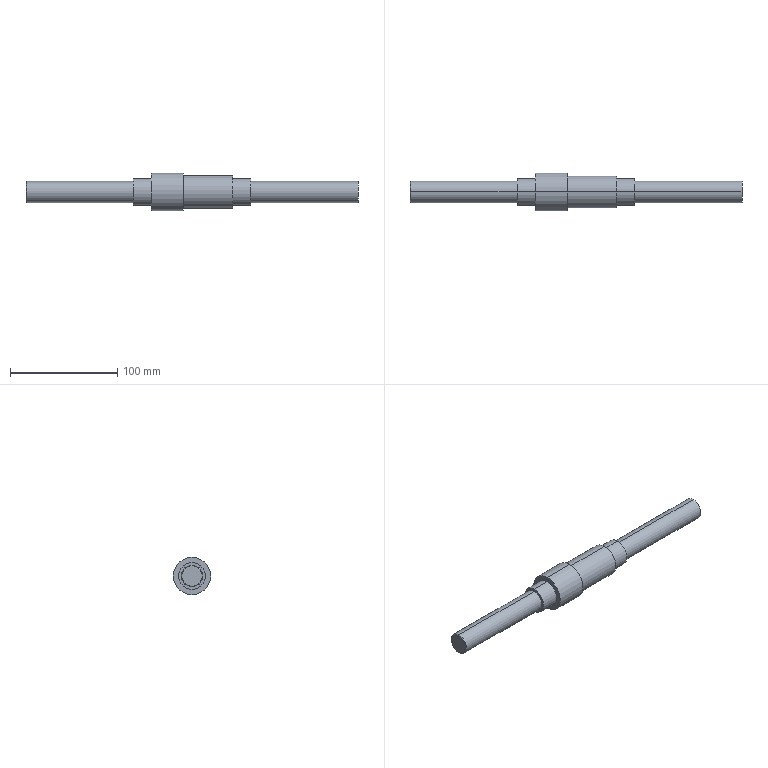Part | STEP file | 1 solid | 21 faces | box 310 x 35 x 35 mm | volume 140893 mm3 | cylinder 12 | plane 7 | cone 2 | commonest cylinder face diameters 20 x4 25 x4 30 x2 35 x2
STEP:
#1=CARTESIAN_POINT('',(0.,0.,0.));
#2=DIRECTION('',(0.,0.,1.));
#3=DIRECTION('',(1.,0.,0.));
#4=AXIS2_PLACEMENT_3D('',#1,#2,#3);
#5=CARTESIAN_POINT('',(210.,0.,-10.));
#6=VERTEX_POINT('',#5);
#7=CARTESIAN_POINT('',(210.,0.,10.));
#8=VERTEX_POINT('',#7);
#9=CARTESIAN_POINT('',(210.,0.,0.));
#10=DIRECTION('',(1.,0.,0.));
#11=DIRECTION('',(0.,0.,-1.));
#12=AXIS2_PLACEMENT_3D('',#9,#10,#11);
#13=CIRCLE('',#12,10.);
#14=CARTESIAN_POINT('',(260.,0.,0.));
#15=DIRECTION('',(1.,0.,0.));
#16=DIRECTION('',(0.,0.,-1.));
#17=AXIS2_PLACEMENT_3D('',#14,#15,#16);
#18=CYLINDRICAL_SURFACE('',#17,10.);
#19=CARTESIAN_POINT('',(0.,-50.));
#20=DIRECTION('',(1.,0.));
#21=VECTOR('',#20,1.);
#22=LINE('',#19,#21);
#23=(GEOMETRIC_REPRESENTATION_CONTEXT(2)PARAMETRIC_REPRESENTATION_CONTEXT()REPRESENTATION_CONTEXT('',''));
#24=DEFINITIONAL_REPRESENTATION('',(#22),#23);
#25=PCURVE('',#18,#24);
#26=CARTESIAN_POINT('',(210.,10.,0.));
#27=DIRECTION('',(1.,0.,0.));
#28=DIRECTION('',(0.,0.,-1.));
#29=AXIS2_PLACEMENT_3D('',#26,#27,#28);
#30=PLANE('',#29);
#31=CARTESIAN_POINT('',(0.,-10.));
#32=DIRECTION('',(1.,0.));
#33=AXIS2_PLACEMENT_2D('',#31,#32);
#34=CIRCLE('',#33,10.);
#35=(GEOMETRIC_REPRESENTATION_CONTEXT(2)PARAMETRIC_REPRESENTATION_CONTEXT()REPRESENTATION_CONTEXT('',''));
#36=DEFINITIONAL_REPRESENTATION('',(#34),#35);
#37=PCURVE('',#30,#36);
#38=SURFACE_CURVE('',#13,(#25,#37),.PCURVE_S1.);
#39=EDGE_CURVE('',#6,#8,#38,.T.);
#40=ORIENTED_EDGE('',*,*,#39,.T.);
#41=CARTESIAN_POINT('',(310.,0.,10.));
#42=VERTEX_POINT('',#41);
#43=CARTESIAN_POINT('',(260.,0.,10.));
#44=DIRECTION('',(1.,0.,0.));
#45=VECTOR('',#44,1.);
#46=LINE('',#43,#45);
#47=CARTESIAN_POINT('',(3.142,0.));
#48=DIRECTION('',(0.,1.));
#49=VECTOR('',#48,1.);
#50=LINE('',#47,#49);
#51=(GEOMETRIC_REPRESENTATION_CONTEXT(2)PARAMETRIC_REPRESENTATION_CONTEXT()REPRESENTATION_CONTEXT('',''));
#52=DEFINITIONAL_REPRESENTATION('',(#50),#51);
#53=PCURVE('',#18,#52);
#54=CARTESIAN_POINT('',(260.,0.,0.));
#55=DIRECTION('',(1.,0.,0.));
#56=DIRECTION('',(0.,0.,-1.));
#57=AXIS2_PLACEMENT_3D('',#54,#55,#56);
#58=CYLINDRICAL_SURFACE('',#57,10.);
#59=CARTESIAN_POINT('',(3.142,0.));
#60=DIRECTION('',(0.,1.));
#61=VECTOR('',#60,1.);
#62=LINE('',#59,#61);
#63=(GEOMETRIC_REPRESENTATION_CONTEXT(2)PARAMETRIC_REPRESENTATION_CONTEXT()REPRESENTATION_CONTEXT('',''));
#64=DEFINITIONAL_REPRESENTATION('',(#62),#63);
#65=PCURVE('',#58,#64);
#66=SURFACE_CURVE('',#46,(#53,#65),.PCURVE_S1.);
#67=EDGE_CURVE('',#8,#42,#66,.T.);
#68=ORIENTED_EDGE('',*,*,#67,.T.);
#69=CARTESIAN_POINT('',(310.,0.,-10.));
#70=VERTEX_POINT('',#69);
#71=CARTESIAN_POINT('',(310.,0.,0.));
#72=DIRECTION('',(-1.,0.,0.));
#73=DIRECTION('',(0.,0.,-1.));
#74=AXIS2_PLACEMENT_3D('',#71,#72,#73);
#75=CIRCLE('',#74,10.);
#76=CARTESIAN_POINT('',(6.283,50.));
#77=DIRECTION('',(-1.,0.));
#78=VECTOR('',#77,1.);
#79=LINE('',#76,#78);
#80=(GEOMETRIC_REPRESENTATION_CONTEXT(2)PARAMETRIC_REPRESENTATION_CONTEXT()REPRESENTATION_CONTEXT('',''));
#81=DEFINITIONAL_REPRESENTATION('',(#79),#80);
#82=PCURVE('',#18,#81);
#83=CARTESIAN_POINT('',(310.,0.,0.));
#84=DIRECTION('',(1.,0.,0.));
#85=DIRECTION('',(0.,0.,-1.));
#86=AXIS2_PLACEMENT_3D('',#83,#84,#85);
#87=PLANE('',#86);
#88=CARTESIAN_POINT('',(10.,0.));
#89=CARTESIAN_POINT('',(10.,-17.321));
#90=CARTESIAN_POINT('',(-5.,-8.66));
#91=CARTESIAN_POINT('',(-20.,0.));
#92=CARTESIAN_POINT('',(-5.,8.66));
#93=CARTESIAN_POINT('',(10.,17.321));
#94=CARTESIAN_POINT('',(10.,0.));
#95=(BOUNDED_CURVE()B_SPLINE_CURVE(2,(#88,#89,#90,#91,#92,#93,#94),.UNSPECIFIED.,.T.,.F.)B_SPLINE_CURVE_WITH_KNOTS((1,2,2,2,2,1),(-2.094,0.,2.094,4.189,6.283,8.378),.UNSPECIFIED.)CURVE()GEOMETRIC_REPRESENTATION_ITEM()RATIONAL_B_SPLINE_CURVE((1.,0.5,1.,0.5,1.,0.5,1.))REPRESENTATION_ITEM(''));
#96=(GEOMETRIC_REPRESENTATION_CONTEXT(2)PARAMETRIC_REPRESENTATION_CONTEXT()REPRESENTATION_CONTEXT('',''));
#97=DEFINITIONAL_REPRESENTATION('',(#95),#96);
#98=PCURVE('',#87,#97);
#99=SURFACE_CURVE('',#75,(#82,#98),.PCURVE_S1.);
#100=EDGE_CURVE('',#42,#70,#99,.T.);
#101=ORIENTED_EDGE('',*,*,#100,.T.);
#102=CARTESIAN_POINT('',(260.,0.,-10.));
#103=DIRECTION('',(1.,0.,0.));
#104=VECTOR('',#103,1.);
#105=LINE('',#102,#104);
#106=CARTESIAN_POINT('',(0.,0.));
#107=DIRECTION('',(0.,1.));
#108=VECTOR('',#107,1.);
#109=LINE('',#106,#108);
#110=(GEOMETRIC_REPRESENTATION_CONTEXT(2)PARAMETRIC_REPRESENTATION_CONTEXT()REPRESENTATION_CONTEXT('',''));
#111=DEFINITIONAL_REPRESENTATION('',(#109),#110);
#112=PCURVE('',#18,#111);
#113=CARTESIAN_POINT('',(6.283,0.));
#114=DIRECTION('',(0.,1.));
#115=VECTOR('',#114,1.);
#116=LINE('',#113,#115);
#117=(GEOMETRIC_REPRESENTATION_CONTEXT(2)PARAMETRIC_REPRESENTATION_CONTEXT()REPRESENTATION_CONTEXT('',''));
#118=DEFINITIONAL_REPRESENTATION('',(#116),#117);
#119=PCURVE('',#58,#118);
#120=SURFACE_CURVE('',#105,(#112,#119),.PCURVE_S1.);
#121=EDGE_CURVE('',#6,#70,#120,.T.);
#122=ORIENTED_EDGE('',*,*,#121,.F.);
#123=EDGE_LOOP('',(#40,#68,#101,#122));
#124=FACE_BOUND('',#123,.T.);
#125=ADVANCED_FACE('',(#124),#18,.T.);
#126=CARTESIAN_POINT('',(193.,0.,-12.5));
#127=VERTEX_POINT('',#126);
#128=CARTESIAN_POINT('',(193.,0.,12.5));
#129=VERTEX_POINT('',#128);
#130=CARTESIAN_POINT('',(193.,0.,0.));
#131=DIRECTION('',(1.,0.,0.));
#132=DIRECTION('',(0.,0.,-1.));
#133=AXIS2_PLACEMENT_3D('',#130,#131,#132);
#134=CIRCLE('',#133,12.5);
#135=CARTESIAN_POINT('',(201.5,0.,0.));
#136=DIRECTION('',(1.,0.,0.));
#137=DIRECTION('',(0.,0.,-1.));
#138=AXIS2_PLACEMENT_3D('',#135,#136,#137);
#139=CYLINDRICAL_SURFACE('',#138,12.5);
#140=CARTESIAN_POINT('',(0.,-8.5));
#141=DIRECTION('',(1.,0.));
#142=VECTOR('',#141,1.);
#143=LINE('',#140,#142);
#144=(GEOMETRIC_REPRESENTATION_CONTEXT(2)PARAMETRIC_REPRESENTATION_CONTEXT()REPRESENTATION_CONTEXT('',''));
#145=DEFINITIONAL_REPRESENTATION('',(#143),#144);
#146=PCURVE('',#139,#145);
#147=CARTESIAN_POINT('',(193.,12.5,0.));
#148=DIRECTION('',(1.,0.,0.));
#149=DIRECTION('',(0.,0.,-1.));
#150=AXIS2_PLACEMENT_3D('',#147,#148,#149);
#151=PLANE('',#150);
#152=CARTESIAN_POINT('',(0.,-12.5));
#153=DIRECTION('',(1.,0.));
#154=AXIS2_PLACEMENT_2D('',#152,#153);
#155=CIRCLE('',#154,12.5);
#156=(GEOMETRIC_REPRESENTATION_CONTEXT(2)PARAMETRIC_REPRESENTATION_CONTEXT()REPRESENTATION_CONTEXT('',''));
#157=DEFINITIONAL_REPRESENTATION('',(#155),#156);
#158=PCURVE('',#151,#157);
#159=SURFACE_CURVE('',#134,(#146,#158),.PCURVE_S1.);
#160=EDGE_CURVE('',#127,#129,#159,.T.);
#161=ORIENTED_EDGE('',*,*,#160,.T.);
#162=CARTESIAN_POINT('',(210.,0.,12.5));
#163=VERTEX_POINT('',#162);
#164=CARTESIAN_POINT('',(201.5,0.,12.5));
#165=DIRECTION('',(1.,0.,0.));
#166=VECTOR('',#165,1.);
#167=LINE('',#164,#166);
#168=CARTESIAN_POINT('',(3.142,0.));
#169=DIRECTION('',(0.,1.));
#170=VECTOR('',#169,1.);
#171=LINE('',#168,#170);
#172=(GEOMETRIC_REPRESENTATION_CONTEXT(2)PARAMETRIC_REPRESENTATION_CONTEXT()REPRESENTATION_CONTEXT('',''));
#173=DEFINITIONAL_REPRESENTATION('',(#171),#172);
#174=PCURVE('',#139,#173);
#175=CARTESIAN_POINT('',(201.5,0.,0.));
#176=DIRECTION('',(1.,0.,0.));
#177=DIRECTION('',(0.,0.,-1.));
#178=AXIS2_PLACEMENT_3D('',#175,#176,#177);
#179=CYLINDRICAL_SURFACE('',#178,12.5);
#180=CARTESIAN_POINT('',(3.142,0.));
#181=DIRECTION('',(0.,1.));
#182=VECTOR('',#181,1.);
#183=LINE('',#180,#182);
#184=(GEOMETRIC_REPRESENTATION_CONTEXT(2)PARAMETRIC_REPRESENTATION_CONTEXT()REPRESENTATION_CONTEXT('',''));
#185=DEFINITIONAL_REPRESENTATION('',(#183),#184);
#186=PCURVE('',#179,#185);
#187=SURFACE_CURVE('',#167,(#174,#186),.PCURVE_S1.);
#188=EDGE_CURVE('',#129,#163,#187,.T.);
#189=ORIENTED_EDGE('',*,*,#188,.T.);
#190=CARTESIAN_POINT('',(210.,0.,-12.5));
#191=VERTEX_POINT('',#190);
#192=CARTESIAN_POINT('',(210.,0.,0.));
#193=DIRECTION('',(1.,0.,0.));
#194=DIRECTION('',(0.,0.,-1.));
#195=AXIS2_PLACEMENT_3D('',#192,#193,#194);
#196=CIRCLE('',#195,12.5);
#197=CARTESIAN_POINT('',(0.,8.5));
#198=DIRECTION('',(1.,0.));
#199=VECTOR('',#198,1.);
#200=LINE('',#197,#199);
#201=(GEOMETRIC_REPRESENTATION_CONTEXT(2)PARAMETRIC_REPRESENTATION_CONTEXT()REPRESENTATION_CONTEXT('',''));
#202=DEFINITIONAL_REPRESENTATION('',(#200),#201);
#203=PCURVE('',#139,#202);
#204=CARTESIAN_POINT('',(0.,-10.));
#205=DIRECTION('',(1.,0.));
#206=AXIS2_PLACEMENT_2D('',#204,#205);
#207=CIRCLE('',#206,12.5);
#208=(GEOMETRIC_REPRESENTATION_CONTEXT(2)PARAMETRIC_REPRESENTATION_CONTEXT()REPRESENTATION_CONTEXT('',''));
#209=DEFINITIONAL_REPRESENTATION('',(#207),#208);
#210=PCURVE('',#30,#209);
#211=SURFACE_CURVE('',#196,(#203,#210),.PCURVE_S1.);
#212=EDGE_CURVE('',#191,#163,#211,.T.);
#213=ORIENTED_EDGE('',*,*,#212,.F.);
#214=CARTESIAN_POINT('',(201.5,0.,-12.5));
#215=DIRECTION('',(1.,0.,0.));
#216=VECTOR('',#215,1.);
#217=LINE('',#214,#216);
#218=CARTESIAN_POINT('',(0.,0.));
#219=DIRECTION('',(0.,1.));
#220=VECTOR('',#219,1.);
#221=LINE('',#218,#220);
#222=(GEOMETRIC_REPRESENTATION_CONTEXT(2)PARAMETRIC_REPRESENTATION_CONTEXT()REPRESENTATION_CONTEXT('',''));
#223=DEFINITIONAL_REPRESENTATION('',(#221),#222);
#224=PCURVE('',#139,#223);
#225=CARTESIAN_POINT('',(6.283,0.));
#226=DIRECTION('',(0.,1.));
#227=VECTOR('',#226,1.);
#228=LINE('',#225,#227);
#229=(GEOMETRIC_REPRESENTATION_CONTEXT(2)PARAMETRIC_REPRESENTATION_CONTEXT()REPRESENTATION_CONTEXT('',''));
#230=DEFINITIONAL_REPRESENTATION('',(#228),#229);
#231=PCURVE('',#179,#230);
#232=SURFACE_CURVE('',#217,(#224,#231),.PCURVE_S1.);
#233=EDGE_CURVE('',#127,#191,#232,.T.);
#234=ORIENTED_EDGE('',*,*,#233,.F.);
#235=EDGE_LOOP('',(#161,#189,#213,#234));
#236=FACE_BOUND('',#235,.T.);
#237=ADVANCED_FACE('',(#236),#139,.T.);
#238=CARTESIAN_POINT('',(147.,0.,-15.));
#239=VERTEX_POINT('',#238);
#240=CARTESIAN_POINT('',(147.,0.,15.));
#241=VERTEX_POINT('',#240);
#242=CARTESIAN_POINT('',(147.,0.,0.));
#243=DIRECTION('',(1.,0.,0.));
#244=DIRECTION('',(0.,0.,-1.));
#245=AXIS2_PLACEMENT_3D('',#242,#243,#244);
#246=CIRCLE('',#245,15.);
#247=CARTESIAN_POINT('',(170.,0.,0.));
#248=DIRECTION('',(1.,0.,0.));
#249=DIRECTION('',(0.,0.,-1.));
#250=AXIS2_PLACEMENT_3D('',#247,#248,#249);
#251=CYLINDRICAL_SURFACE('',#250,15.);
#252=CARTESIAN_POINT('',(0.,-23.));
#253=DIRECTION('',(1.,0.));
#254=VECTOR('',#253,1.);
#255=LINE('',#252,#254);
#256=(GEOMETRIC_REPRESENTATION_CONTEXT(2)PARAMETRIC_REPRESENTATION_CONTEXT()REPRESENTATION_CONTEXT('',''));
#257=DEFINITIONAL_REPRESENTATION('',(#255),#256);
#258=PCURVE('',#251,#257);
#259=CARTESIAN_POINT('',(147.,15.,0.));
#260=DIRECTION('',(1.,0.,0.));
#261=DIRECTION('',(0.,0.,-1.));
#262=AXIS2_PLACEMENT_3D('',#259,#260,#261);
#263=PLANE('',#262);
#264=CARTESIAN_POINT('',(0.,-15.));
#265=DIRECTION('',(1.,0.));
#266=AXIS2_PLACEMENT_2D('',#264,#265);
#267=CIRCLE('',#266,15.);
#268=(GEOMETRIC_REPRESENTATION_CONTEXT(2)PARAMETRIC_REPRESENTATION_CONTEXT()REPRESENTATION_CONTEXT('',''));
#269=DEFINITIONAL_REPRESENTATION('',(#267),#268);
#270=PCURVE('',#263,#269);
#271=SURFACE_CURVE('',#246,(#258,#270),.PCURVE_S1.);
#272=EDGE_CURVE('',#239,#241,#271,.T.);
#273=ORIENTED_EDGE('',*,*,#272,.T.);
#274=CARTESIAN_POINT('',(193.,0.,15.));
#275=VERTEX_POINT('',#274);
#276=CARTESIAN_POINT('',(170.,0.,15.));
#277=DIRECTION('',(1.,0.,0.));
#278=VECTOR('',#277,1.);
#279=LINE('',#276,#278);
#280=CARTESIAN_POINT('',(3.142,0.));
#281=DIRECTION('',(0.,1.));
#282=VECTOR('',#281,1.);
#283=LINE('',#280,#282);
#284=(GEOMETRIC_REPRESENTATION_CONTEXT(2)PARAMETRIC_REPRESENTATION_CONTEXT()REPRESENTATION_CONTEXT('',''));
#285=DEFINITIONAL_REPRESENTATION('',(#283),#284);
#286=PCURVE('',#251,#285);
#287=CARTESIAN_POINT('',(170.,0.,0.));
#288=DIRECTION('',(1.,0.,0.));
#289=DIRECTION('',(0.,0.,-1.));
#290=AXIS2_PLACEMENT_3D('',#287,#288,#289);
#291=CYLINDRICAL_SURFACE('',#290,15.);
#292=CARTESIAN_POINT('',(3.142,0.));
#293=DIRECTION('',(0.,1.));
#294=VECTOR('',#293,1.);
#295=LINE('',#292,#294);
#296=(GEOMETRIC_REPRESENTATION_CONTEXT(2)PARAMETRIC_REPRESENTATION_CONTEXT()REPRESENTATION_CONTEXT('',''));
#297=DEFINITIONAL_REPRESENTATION('',(#295),#296);
#298=PCURVE('',#291,#297);
#299=SURFACE_CURVE('',#279,(#286,#298),.PCURVE_S1.);
#300=EDGE_CURVE('',#241,#275,#299,.T.);
#301=ORIENTED_EDGE('',*,*,#300,.T.);
#302=CARTESIAN_POINT('',(193.,0.,-15.));
#303=VERTEX_POINT('',#302);
#304=CARTESIAN_POINT('',(193.,0.,0.));
#305=DIRECTION('',(1.,0.,0.));
#306=DIRECTION('',(0.,0.,-1.));
#307=AXIS2_PLACEMENT_3D('',#304,#305,#306);
#308=CIRCLE('',#307,15.);
#309=CARTESIAN_POINT('',(0.,23.));
#310=DIRECTION('',(1.,0.));
#311=VECTOR('',#310,1.);
#312=LINE('',#309,#311);
#313=(GEOMETRIC_REPRESENTATION_CONTEXT(2)PARAMETRIC_REPRESENTATION_CONTEXT()REPRESENTATION_CONTEXT('',''));
#314=DEFINITIONAL_REPRESENTATION('',(#312),#313);
#315=PCURVE('',#251,#314);
#316=CARTESIAN_POINT('',(0.,-12.5));
#317=DIRECTION('',(1.,0.));
#318=AXIS2_PLACEMENT_2D('',#316,#317);
#319=CIRCLE('',#318,15.);
#320=(GEOMETRIC_REPRESENTATION_CONTEXT(2)PARAMETRIC_REPRESENTATION_CONTEXT()REPRESENTATION_CONTEXT('',''));
#321=DEFINITIONAL_REPRESENTATION('',(#319),#320);
#322=PCURVE('',#151,#321);
#323=SURFACE_CURVE('',#308,(#315,#322),.PCURVE_S1.);
#324=EDGE_CURVE('',#303,#275,#323,.T.);
#325=ORIENTED_EDGE('',*,*,#324,.F.);
#326=CARTESIAN_POINT('',(170.,0.,-15.));
#327=DIRECTION('',(1.,0.,0.));
#328=VECTOR('',#327,1.);
#329=LINE('',#326,#328);
#330=CARTESIAN_POINT('',(0.,0.));
#331=DIRECTION('',(0.,1.));
#332=VECTOR('',#331,1.);
#333=LINE('',#330,#332);
#334=(GEOMETRIC_REPRESENTATION_CONTEXT(2)PARAMETRIC_REPRESENTATION_CONTEXT()REPRESENTATION_CONTEXT('',''));
#335=DEFINITIONAL_REPRESENTATION('',(#333),#334);
#336=PCURVE('',#251,#335);
#337=CARTESIAN_POINT('',(6.283,0.));
#338=DIRECTION('',(0.,1.));
#339=VECTOR('',#338,1.);
#340=LINE('',#337,#339);
#341=(GEOMETRIC_REPRESENTATION_CONTEXT(2)PARAMETRIC_REPRESENTATION_CONTEXT()REPRESENTATION_CONTEXT('',''));
#342=DEFINITIONAL_REPRESENTATION('',(#340),#341);
#343=PCURVE('',#291,#342);
#344=SURFACE_CURVE('',#329,(#336,#343),.PCURVE_S1.);
#345=EDGE_CURVE('',#239,#303,#344,.T.);
#346=ORIENTED_EDGE('',*,*,#345,.F.);
#347=EDGE_LOOP('',(#273,#301,#325,#346));
#348=FACE_BOUND('',#347,.T.);
#349=ADVANCED_FACE('',(#348),#251,.T.);
#350=CARTESIAN_POINT('',(117.,0.,-17.5));
#351=VERTEX_POINT('',#350);
#352=CARTESIAN_POINT('',(117.,0.,17.5));
#353=VERTEX_POINT('',#352);
#354=CARTESIAN_POINT('',(117.,0.,0.));
#355=DIRECTION('',(1.,0.,0.));
#356=DIRECTION('',(0.,0.,-1.));
#357=AXIS2_PLACEMENT_3D('',#354,#355,#356);
#358=CIRCLE('',#357,17.5);
#359=CARTESIAN_POINT('',(132.,0.,0.));
#360=DIRECTION('',(1.,0.,0.));
#361=DIRECTION('',(0.,0.,-1.));
#362=AXIS2_PLACEMENT_3D('',#359,#360,#361);
#363=CYLINDRICAL_SURFACE('',#362,17.5);
#364=CARTESIAN_POINT('',(0.,-15.));
#365=DIRECTION('',(1.,0.));
#366=VECTOR('',#365,1.);
#367=LINE('',#364,#366);
#368=(GEOMETRIC_REPRESENTATION_CONTEXT(2)PARAMETRIC_REPRESENTATION_CONTEXT()REPRESENTATION_CONTEXT('',''));
#369=DEFINITIONAL_REPRESENTATION('',(#367),#368);
#370=PCURVE('',#363,#369);
#371=CARTESIAN_POINT('',(117.,17.5,0.));
#372=DIRECTION('',(-1.,0.,0.));
#373=DIRECTION('',(0.,0.,1.));
#374=AXIS2_PLACEMENT_3D('',#371,#372,#373);
#375=PLANE('',#374);
#376=CARTESIAN_POINT('',(-17.5,-17.5));
#377=CARTESIAN_POINT('',(-17.5,12.811));
#378=CARTESIAN_POINT('',(8.75,-2.345));
#379=CARTESIAN_POINT('',(35.,-17.5));
#380=CARTESIAN_POINT('',(8.75,-32.655));
#381=CARTESIAN_POINT('',(-17.5,-47.811));
#382=CARTESIAN_POINT('',(-17.5,-17.5));
#383=(BOUNDED_CURVE()B_SPLINE_CURVE(2,(#376,#377,#378,#379,#380,#381,#382),.UNSPECIFIED.,.T.,.F.)B_SPLINE_CURVE_WITH_KNOTS((1,2,2,2,2,1),(-2.094,0.,2.094,4.189,6.283,8.378),.UNSPECIFIED.)CURVE()GEOMETRIC_REPRESENTATION_ITEM()RATIONAL_B_SPLINE_CURVE((1.,0.5,1.,0.5,1.,0.5,1.))REPRESENTATION_ITEM(''));
#384=(GEOMETRIC_REPRESENTATION_CONTEXT(2)PARAMETRIC_REPRESENTATION_CONTEXT()REPRESENTATION_CONTEXT('',''));
#385=DEFINITIONAL_REPRESENTATION('',(#383),#384);
#386=PCURVE('',#375,#385);
#387=SURFACE_CURVE('',#358,(#370,#386),.PCURVE_S1.);
#388=EDGE_CURVE('',#351,#353,#387,.T.);
#389=ORIENTED_EDGE('',*,*,#388,.T.);
#390=CARTESIAN_POINT('',(147.,0.,17.5));
#391=VERTEX_POINT('',#390);
#392=CARTESIAN_POINT('',(132.,0.,17.5));
#393=DIRECTION('',(1.,0.,0.));
#394=VECTOR('',#393,1.);
#395=LINE('',#392,#394);
#396=CARTESIAN_POINT('',(3.142,0.));
#397=DIRECTION('',(0.,1.));
#398=VECTOR('',#397,1.);
#399=LINE('',#396,#398);
#400=(GEOMETRIC_REPRESENTATION_CONTEXT(2)PARAMETRIC_REPRESENTATION_CONTEXT()REPRESENTATION_CONTEXT('',''));
#401=DEFINITIONAL_REPRESENTATION('',(#399),#400);
#402=PCURVE('',#363,#401);
#403=CARTESIAN_POINT('',(132.,0.,0.));
#404=DIRECTION('',(1.,0.,0.));
#405=DIRECTION('',(0.,0.,-1.));
#406=AXIS2_PLACEMENT_3D('',#403,#404,#405);
#407=CYLINDRICAL_SURFACE('',#406,17.5);
#408=CARTESIAN_POINT('',(3.142,0.));
#409=DIRECTION('',(0.,1.));
#410=VECTOR('',#409,1.);
#411=LINE('',#408,#410);
#412=(GEOMETRIC_REPRESENTATION_CONTEXT(2)PARAMETRIC_REPRESENTATION_CONTEXT()REPRESENTATION_CONTEXT('',''));
#413=DEFINITIONAL_REPRESENTATION('',(#411),#412);
#414=PCURVE('',#407,#413);
#415=SURFACE_CURVE('',#395,(#402,#414),.PCURVE_S1.);
#416=EDGE_CURVE('',#353,#391,#415,.T.);
#417=ORIENTED_EDGE('',*,*,#416,.T.);
#418=CARTESIAN_POINT('',(147.,0.,-17.5));
#419=VERTEX_POINT('',#418);
#420=CARTESIAN_POINT('',(147.,0.,0.));
#421=DIRECTION('',(1.,0.,0.));
#422=DIRECTION('',(0.,0.,-1.));
#423=AXIS2_PLACEMENT_3D('',#420,#421,#422);
#424=CIRCLE('',#423,17.5);
#425=CARTESIAN_POINT('',(0.,15.));
#426=DIRECTION('',(1.,0.));
#427=VECTOR('',#426,1.);
#428=LINE('',#425,#427);
#429=(GEOMETRIC_REPRESENTATION_CONTEXT(2)PARAMETRIC_REPRESENTATION_CONTEXT()REPRESENTATION_CONTEXT('',''));
#430=DEFINITIONAL_REPRESENTATION('',(#428),#429);
#431=PCURVE('',#363,#430);
#432=CARTESIAN_POINT('',(0.,-15.));
#433=DIRECTION('',(1.,0.));
#434=AXIS2_PLACEMENT_2D('',#432,#433);
#435=CIRCLE('',#434,17.5);
#436=(GEOMETRIC_REPRESENTATION_CONTEXT(2)PARAMETRIC_REPRESENTATION_CONTEXT()REPRESENTATION_CONTEXT('',''));
#437=DEFINITIONAL_REPRESENTATION('',(#435),#436);
#438=PCURVE('',#263,#437);
#439=SURFACE_CURVE('',#424,(#431,#438),.PCURVE_S1.);
#440=EDGE_CURVE('',#419,#391,#439,.T.);
#441=ORIENTED_EDGE('',*,*,#440,.F.);
#442=CARTESIAN_POINT('',(132.,0.,-17.5));
#443=DIRECTION('',(1.,0.,0.));
#444=VECTOR('',#443,1.);
#445=LINE('',#442,#444);
#446=CARTESIAN_POINT('',(0.,0.));
#447=DIRECTION('',(0.,1.));
#448=VECTOR('',#447,1.);
#449=LINE('',#446,#448);
#450=(GEOMETRIC_REPRESENTATION_CONTEXT(2)PARAMETRIC_REPRESENTATION_CONTEXT()REPRESENTATION_CONTEXT('',''));
#451=DEFINITIONAL_REPRESENTATION('',(#449),#450);
#452=PCURVE('',#363,#451);
#453=CARTESIAN_POINT('',(6.283,0.));
#454=DIRECTION('',(0.,1.));
#455=VECTOR('',#454,1.);
#456=LINE('',#453,#455);
#457=(GEOMETRIC_REPRESENTATION_CONTEXT(2)PARAMETRIC_REPRESENTATION_CONTEXT()REPRESENTATION_CONTEXT('',''));
#458=DEFINITIONAL_REPRESENTATION('',(#456),#457);
#459=PCURVE('',#407,#458);
#460=SURFACE_CURVE('',#445,(#452,#459),.PCURVE_S1.);
#461=EDGE_CURVE('',#351,#419,#460,.T.);
#462=ORIENTED_EDGE('',*,*,#461,.F.);
#463=EDGE_LOOP('',(#389,#417,#441,#462));
#464=FACE_BOUND('',#463,.T.);
#465=ADVANCED_FACE('',(#464),#363,.T.);
#466=CARTESIAN_POINT('',(100.,0.,-12.5));
#467=VERTEX_POINT('',#466);
#468=CARTESIAN_POINT('',(100.,0.,12.5));
#469=VERTEX_POINT('',#468);
#470=CARTESIAN_POINT('',(100.,0.,0.));
#471=DIRECTION('',(1.,0.,0.));
#472=DIRECTION('',(0.,0.,-1.));
#473=AXIS2_PLACEMENT_3D('',#470,#471,#472);
#474=CIRCLE('',#473,12.5);
#475=CARTESIAN_POINT('',(108.5,0.,0.));
#476=DIRECTION('',(1.,0.,0.));
#477=DIRECTION('',(0.,0.,-1.));
#478=AXIS2_PLACEMENT_3D('',#475,#476,#477);
#479=CYLINDRICAL_SURFACE('',#478,12.5);
#480=CARTESIAN_POINT('',(0.,-8.5));
#481=DIRECTION('',(1.,0.));
#482=VECTOR('',#481,1.);
#483=LINE('',#480,#482);
#484=(GEOMETRIC_REPRESENTATION_CONTEXT(2)PARAMETRIC_REPRESENTATION_CONTEXT()REPRESENTATION_CONTEXT('',''));
#485=DEFINITIONAL_REPRESENTATION('',(#483),#484);
#486=PCURVE('',#479,#485);
#487=CARTESIAN_POINT('',(100.,12.5,0.));
#488=DIRECTION('',(-1.,0.,0.));
#489=DIRECTION('',(0.,0.,1.));
#490=AXIS2_PLACEMENT_3D('',#487,#488,#489);
#491=PLANE('',#490);
#492=CARTESIAN_POINT('',(-12.5,-12.5));
#493=CARTESIAN_POINT('',(-12.5,9.151));
#494=CARTESIAN_POINT('',(6.25,-1.675));
#495=CARTESIAN_POINT('',(25.,-12.5));
#496=CARTESIAN_POINT('',(6.25,-23.325));
#497=CARTESIAN_POINT('',(-12.5,-34.151));
#498=CARTESIAN_POINT('',(-12.5,-12.5));
#499=(BOUNDED_CURVE()B_SPLINE_CURVE(2,(#492,#493,#494,#495,#496,#497,#498),.UNSPECIFIED.,.T.,.F.)B_SPLINE_CURVE_WITH_KNOTS((1,2,2,2,2,1),(-2.094,0.,2.094,4.189,6.283,8.378),.UNSPECIFIED.)CURVE()GEOMETRIC_REPRESENTATION_ITEM()RATIONAL_B_SPLINE_CURVE((1.,0.5,1.,0.5,1.,0.5,1.))REPRESENTATION_ITEM(''));
#500=(GEOMETRIC_REPRESENTATION_CONTEXT(2)PARAMETRIC_REPRESENTATION_CONTEXT()REPRESENTATION_CONTEXT('',''));
#501=DEFINITIONAL_REPRESENTATION('',(#499),#500);
#502=PCURVE('',#491,#501);
#503=SURFACE_CURVE('',#474,(#486,#502),.PCURVE_S1.);
#504=EDGE_CURVE('',#467,#469,#503,.T.);
#505=ORIENTED_EDGE('',*,*,#504,.T.);
#506=CARTESIAN_POINT('',(117.,0.,12.5));
#507=VERTEX_POINT('',#506);
#508=CARTESIAN_POINT('',(108.5,0.,12.5));
#509=DIRECTION('',(1.,0.,0.));
#510=VECTOR('',#509,1.);
#511=LINE('',#508,#510);
#512=CARTESIAN_POINT('',(3.142,0.));
#513=DIRECTION('',(0.,1.));
#514=VECTOR('',#513,1.);
#515=LINE('',#512,#514);
#516=(GEOMETRIC_REPRESENTATION_CONTEXT(2)PARAMETRIC_REPRESENTATION_CONTEXT()REPRESENTATION_CONTEXT('',''));
#517=DEFINITIONAL_REPRESENTATION('',(#515),#516);
#518=PCURVE('',#479,#517);
#519=CARTESIAN_POINT('',(108.5,0.,0.));
#520=DIRECTION('',(1.,0.,0.));
#521=DIRECTION('',(0.,0.,-1.));
#522=AXIS2_PLACEMENT_3D('',#519,#520,#521);
#523=CYLINDRICAL_SURFACE('',#522,12.5);
#524=CARTESIAN_POINT('',(3.142,0.));
#525=DIRECTION('',(0.,1.));
#526=VECTOR('',#525,1.);
#527=LINE('',#524,#526);
#528=(GEOMETRIC_REPRESENTATION_CONTEXT(2)PARAMETRIC_REPRESENTATION_CONTEXT()REPRESENTATION_CONTEXT('',''));
#529=DEFINITIONAL_REPRESENTATION('',(#527),#528);
#530=PCURVE('',#523,#529);
#531=SURFACE_CURVE('',#511,(#518,#530),.PCURVE_S1.);
#532=EDGE_CURVE('',#469,#507,#531,.T.);
#533=ORIENTED_EDGE('',*,*,#532,.T.);
#534=CARTESIAN_POINT('',(117.,0.,-12.5));
#535=VERTEX_POINT('',#534);
#536=CARTESIAN_POINT('',(117.,0.,0.));
#537=DIRECTION('',(1.,0.,0.));
#538=DIRECTION('',(0.,0.,-1.));
#539=AXIS2_PLACEMENT_3D('',#536,#537,#538);
#540=CIRCLE('',#539,12.5);
#541=CARTESIAN_POINT('',(0.,8.5));
#542=DIRECTION('',(1.,0.));
#543=VECTOR('',#542,1.);
#544=LINE('',#541,#543);
#545=(GEOMETRIC_REPRESENTATION_CONTEXT(2)PARAMETRIC_REPRESENTATION_CONTEXT()REPRESENTATION_CONTEXT('',''));
#546=DEFINITIONAL_REPRESENTATION('',(#544),#545);
#547=PCURVE('',#479,#546);
#548=CARTESIAN_POINT('',(-12.5,-17.5));
#549=CARTESIAN_POINT('',(-12.5,4.151));
#550=CARTESIAN_POINT('',(6.25,-6.675));
#551=CARTESIAN_POINT('',(25.,-17.5));
#552=CARTESIAN_POINT('',(6.25,-28.325));
#553=CARTESIAN_POINT('',(-12.5,-39.151));
#554=CARTESIAN_POINT('',(-12.5,-17.5));
#555=(BOUNDED_CURVE()B_SPLINE_CURVE(2,(#548,#549,#550,#551,#552,#553,#554),.UNSPECIFIED.,.T.,.F.)B_SPLINE_CURVE_WITH_KNOTS((1,2,2,2,2,1),(-2.094,0.,2.094,4.189,6.283,8.378),.UNSPECIFIED.)CURVE()GEOMETRIC_REPRESENTATION_ITEM()RATIONAL_B_SPLINE_CURVE((1.,0.5,1.,0.5,1.,0.5,1.))REPRESENTATION_ITEM(''));
#556=(GEOMETRIC_REPRESENTATION_CONTEXT(2)PARAMETRIC_REPRESENTATION_CONTEXT()REPRESENTATION_CONTEXT('',''));
#557=DEFINITIONAL_REPRESENTATION('',(#555),#556);
#558=PCURVE('',#375,#557);
#559=SURFACE_CURVE('',#540,(#547,#558),.PCURVE_S1.);
#560=EDGE_CURVE('',#535,#507,#559,.T.);
#561=ORIENTED_EDGE('',*,*,#560,.F.);
#562=CARTESIAN_POINT('',(108.5,0.,-12.5));
#563=DIRECTION('',(1.,0.,0.));
#564=VECTOR('',#563,1.);
#565=LINE('',#562,#564);
#566=CARTESIAN_POINT('',(0.,0.));
#567=DIRECTION('',(0.,1.));
#568=VECTOR('',#567,1.);
#569=LINE('',#566,#568);
#570=(GEOMETRIC_REPRESENTATION_CONTEXT(2)PARAMETRIC_REPRESENTATION_CONTEXT()REPRESENTATION_CONTEXT('',''));
#571=DEFINITIONAL_REPRESENTATION('',(#569),#570);
#572=PCURVE('',#479,#571);
#573=CARTESIAN_POINT('',(6.283,0.));
#574=DIRECTION('',(0.,1.));
#575=VECTOR('',#574,1.);
#576=LINE('',#573,#575);
#577=(GEOMETRIC_REPRESENTATION_CONTEXT(2)PARAMETRIC_REPRESENTATION_CONTEXT()REPRESENTATION_CONTEXT('',''));
#578=DEFINITIONAL_REPRESENTATION('',(#576),#577);
#579=PCURVE('',#523,#578);
#580=SURFACE_CURVE('',#565,(#572,#579),.PCURVE_S1.);
#581=EDGE_CURVE('',#467,#535,#580,.T.);
#582=ORIENTED_EDGE('',*,*,#581,.F.);
#583=EDGE_LOOP('',(#505,#533,#561,#582));
#584=FACE_BOUND('',#583,.T.);
#585=ADVANCED_FACE('',(#584),#479,.T.);
#586=CARTESIAN_POINT('',(0.5,0.,-10.));
#587=VERTEX_POINT('',#586);
#588=CARTESIAN_POINT('',(0.5,0.,10.));
#589=VERTEX_POINT('',#588);
#590=CARTESIAN_POINT('',(0.5,0.,0.));
#591=DIRECTION('',(1.,0.,0.));
#592=DIRECTION('',(0.,0.,-1.));
#593=AXIS2_PLACEMENT_3D('',#590,#591,#592);
#594=CIRCLE('',#593,10.);
#595=CARTESIAN_POINT('',(50.,0.,0.));
#596=DIRECTION('',(1.,0.,0.));
#597=DIRECTION('',(0.,0.,-1.));
#598=AXIS2_PLACEMENT_3D('',#595,#596,#597);
#599=CYLINDRICAL_SURFACE('',#598,10.);
#600=CARTESIAN_POINT('',(0.,-49.5));
#601=DIRECTION('',(1.,0.));
#602=VECTOR('',#601,1.);
#603=LINE('',#600,#602);
#604=(GEOMETRIC_REPRESENTATION_CONTEXT(2)PARAMETRIC_REPRESENTATION_CONTEXT()REPRESENTATION_CONTEXT('',''));
#605=DEFINITIONAL_REPRESENTATION('',(#603),#604);
#606=PCURVE('',#599,#605);
#607=CARTESIAN_POINT('',(0.5,0.,0.));
#608=DIRECTION('',(1.,0.,0.));
#609=DIRECTION('',(0.,0.,-1.));
#610=AXIS2_PLACEMENT_3D('',#607,#608,#609);
#611=CONICAL_SURFACE('',#610,10.,0.7854);
#612=CARTESIAN_POINT('',(0.,0.));
#613=DIRECTION('',(1.,0.));
#614=VECTOR('',#613,1.);
#615=LINE('',#612,#614);
#616=(GEOMETRIC_REPRESENTATION_CONTEXT(2)PARAMETRIC_REPRESENTATION_CONTEXT()REPRESENTATION_CONTEXT('',''));
#617=DEFINITIONAL_REPRESENTATION('',(#615),#616);
#618=PCURVE('',#611,#617);
#619=SURFACE_CURVE('',#594,(#606,#618),.PCURVE_S1.);
#620=EDGE_CURVE('',#587,#589,#619,.T.);
#621=ORIENTED_EDGE('',*,*,#620,.T.);
#622=CARTESIAN_POINT('',(100.,0.,10.));
#623=VERTEX_POINT('',#622);
#624=CARTESIAN_POINT('',(50.,0.,10.));
#625=DIRECTION('',(1.,0.,0.));
#626=VECTOR('',#625,1.);
#627=LINE('',#624,#626);
#628=CARTESIAN_POINT('',(3.142,0.));
#629=DIRECTION('',(0.,1.));
#630=VECTOR('',#629,1.);
#631=LINE('',#628,#630);
#632=(GEOMETRIC_REPRESENTATION_CONTEXT(2)PARAMETRIC_REPRESENTATION_CONTEXT()REPRESENTATION_CONTEXT('',''));
#633=DEFINITIONAL_REPRESENTATION('',(#631),#632);
#634=PCURVE('',#599,#633);
#635=CARTESIAN_POINT('',(50.,0.,0.));
#636=DIRECTION('',(1.,0.,0.));
#637=DIRECTION('',(0.,0.,-1.));
#638=AXIS2_PLACEMENT_3D('',#635,#636,#637);
#639=CYLINDRICAL_SURFACE('',#638,10.);
#640=CARTESIAN_POINT('',(3.142,0.));
#641=DIRECTION('',(0.,1.));
#642=VECTOR('',#641,1.);
#643=LINE('',#640,#642);
#644=(GEOMETRIC_REPRESENTATION_CONTEXT(2)PARAMETRIC_REPRESENTATION_CONTEXT()REPRESENTATION_CONTEXT('',''));
#645=DEFINITIONAL_REPRESENTATION('',(#643),#644);
#646=PCURVE('',#639,#645);
#647=SURFACE_CURVE('',#627,(#634,#646),.PCURVE_S1.);
#648=EDGE_CURVE('',#589,#623,#647,.T.);
#649=ORIENTED_EDGE('',*,*,#648,.T.);
#650=CARTESIAN_POINT('',(100.,0.,-10.));
#651=VERTEX_POINT('',#650);
#652=CARTESIAN_POINT('',(100.,0.,0.));
#653=DIRECTION('',(1.,0.,0.));
#654=DIRECTION('',(0.,0.,-1.));
#655=AXIS2_PLACEMENT_3D('',#652,#653,#654);
#656=CIRCLE('',#655,10.);
#657=CARTESIAN_POINT('',(0.,50.));
#658=DIRECTION('',(1.,0.));
#659=VECTOR('',#658,1.);
#660=LINE('',#657,#659);
#661=(GEOMETRIC_REPRESENTATION_CONTEXT(2)PARAMETRIC_REPRESENTATION_CONTEXT()REPRESENTATION_CONTEXT('',''));
#662=DEFINITIONAL_REPRESENTATION('',(#660),#661);
#663=PCURVE('',#599,#662);
#664=CARTESIAN_POINT('',(-10.,-12.5));
#665=CARTESIAN_POINT('',(-10.,4.821));
#666=CARTESIAN_POINT('',(5.,-3.84));
#667=CARTESIAN_POINT('',(20.,-12.5));
#668=CARTESIAN_POINT('',(5.,-21.16));
#669=CARTESIAN_POINT('',(-10.,-29.821));
#670=CARTESIAN_POINT('',(-10.,-12.5));
#671=(BOUNDED_CURVE()B_SPLINE_CURVE(2,(#664,#665,#666,#667,#668,#669,#670),.UNSPECIFIED.,.T.,.F.)B_SPLINE_CURVE_WITH_KNOTS((1,2,2,2,2,1),(-2.094,0.,2.094,4.189,6.283,8.378),.UNSPECIFIED.)CURVE()GEOMETRIC_REPRESENTATION_ITEM()RATIONAL_B_SPLINE_CURVE((1.,0.5,1.,0.5,1.,0.5,1.))REPRESENTATION_ITEM(''));
#672=(GEOMETRIC_REPRESENTATION_CONTEXT(2)PARAMETRIC_REPRESENTATION_CONTEXT()REPRESENTATION_CONTEXT('',''));
#673=DEFINITIONAL_REPRESENTATION('',(#671),#672);
#674=PCURVE('',#491,#673);
#675=SURFACE_CURVE('',#656,(#663,#674),.PCURVE_S1.);
#676=EDGE_CURVE('',#651,#623,#675,.T.);
#677=ORIENTED_EDGE('',*,*,#676,.F.);
#678=CARTESIAN_POINT('',(50.,0.,-10.));
#679=DIRECTION('',(1.,0.,0.));
#680=VECTOR('',#679,1.);
#681=LINE('',#678,#680);
#682=CARTESIAN_POINT('',(0.,0.));
#683=DIRECTION('',(0.,1.));
#684=VECTOR('',#683,1.);
#685=LINE('',#682,#684);
#686=(GEOMETRIC_REPRESENTATION_CONTEXT(2)PARAMETRIC_REPRESENTATION_CONTEXT()REPRESENTATION_CONTEXT('',''));
#687=DEFINITIONAL_REPRESENTATION('',(#685),#686);
#688=PCURVE('',#599,#687);
#689=CARTESIAN_POINT('',(6.283,0.));
#690=DIRECTION('',(0.,1.));
#691=VECTOR('',#690,1.);
#692=LINE('',#689,#691);
#693=(GEOMETRIC_REPRESENTATION_CONTEXT(2)PARAMETRIC_REPRESENTATION_CONTEXT()REPRESENTATION_CONTEXT('',''));
#694=DEFINITIONAL_REPRESENTATION('',(#692),#693);
#695=PCURVE('',#639,#694);
#696=SURFACE_CURVE('',#681,(#688,#695),.PCURVE_S1.);
#697=EDGE_CURVE('',#587,#651,#696,.T.);
#698=ORIENTED_EDGE('',*,*,#697,.F.);
#699=EDGE_LOOP('',(#621,#649,#677,#698));
#700=FACE_BOUND('',#699,.T.);
#701=ADVANCED_FACE('',(#700),#599,.T.);
#702=CARTESIAN_POINT('',(0.,0.,-9.5));
#703=VERTEX_POINT('',#702);
#704=CARTESIAN_POINT('',(0.,0.,9.5));
#705=VERTEX_POINT('',#704);
#706=CARTESIAN_POINT('',(0.,0.,0.));
#707=DIRECTION('',(1.,0.,0.));
#708=DIRECTION('',(0.,0.,-1.));
#709=AXIS2_PLACEMENT_3D('',#706,#707,#708);
#710=CIRCLE('',#709,9.5);
#711=CARTESIAN_POINT('',(0.,-0.5));
#712=DIRECTION('',(1.,0.));
#713=VECTOR('',#712,1.);
#714=LINE('',#711,#713);
#715=(GEOMETRIC_REPRESENTATION_CONTEXT(2)PARAMETRIC_REPRESENTATION_CONTEXT()REPRESENTATION_CONTEXT('',''));
#716=DEFINITIONAL_REPRESENTATION('',(#714),#715);
#717=PCURVE('',#611,#716);
#718=CARTESIAN_POINT('',(0.,10.,0.));
#719=DIRECTION('',(-1.,0.,0.));
#720=DIRECTION('',(0.,0.,1.));
#721=AXIS2_PLACEMENT_3D('',#718,#719,#720);
#722=PLANE('',#721);
#723=CARTESIAN_POINT('',(-9.5,-10.));
#724=CARTESIAN_POINT('',(-9.5,6.454));
#725=CARTESIAN_POINT('',(4.75,-1.773));
#726=CARTESIAN_POINT('',(19.,-10.));
#727=CARTESIAN_POINT('',(4.75,-18.227));
#728=CARTESIAN_POINT('',(-9.5,-26.454));
#729=CARTESIAN_POINT('',(-9.5,-10.));
#730=(BOUNDED_CURVE()B_SPLINE_CURVE(2,(#723,#724,#725,#726,#727,#728,#729),.UNSPECIFIED.,.T.,.F.)B_SPLINE_CURVE_WITH_KNOTS((1,2,2,2,2,1),(-2.094,0.,2.094,4.189,6.283,8.378),.UNSPECIFIED.)CURVE()GEOMETRIC_REPRESENTATION_ITEM()RATIONAL_B_SPLINE_CURVE((1.,0.5,1.,0.5,1.,0.5,1.))REPRESENTATION_ITEM(''));
#731=(GEOMETRIC_REPRESENTATION_CONTEXT(2)PARAMETRIC_REPRESENTATION_CONTEXT()REPRESENTATION_CONTEXT('',''));
#732=DEFINITIONAL_REPRESENTATION('',(#730),#731);
#733=PCURVE('',#722,#732);
#734=SURFACE_CURVE('',#710,(#717,#733),.PCURVE_S1.);
#735=EDGE_CURVE('',#703,#705,#734,.T.);
#736=ORIENTED_EDGE('',*,*,#735,.T.);
#737=CARTESIAN_POINT('',(0.5,0.,10.));
#738=DIRECTION('',(0.7071,0.,0.7071));
#739=VECTOR('',#738,1.);
#740=LINE('',#737,#739);
#741=CARTESIAN_POINT('',(3.142,0.));
#742=DIRECTION('',(0.,1.));
#743=VECTOR('',#742,1.);
#744=LINE('',#741,#743);
#745=(GEOMETRIC_REPRESENTATION_CONTEXT(2)PARAMETRIC_REPRESENTATION_CONTEXT()REPRESENTATION_CONTEXT('',''));
#746=DEFINITIONAL_REPRESENTATION('',(#744),#745);
#747=PCURVE('',#611,#746);
#748=CARTESIAN_POINT('',(0.5,0.,0.));
#749=DIRECTION('',(1.,0.,0.));
#750=DIRECTION('',(0.,0.,-1.));
#751=AXIS2_PLACEMENT_3D('',#748,#749,#750);
#752=CONICAL_SURFACE('',#751,10.,0.7854);
#753=CARTESIAN_POINT('',(3.142,0.));
#754=DIRECTION('',(0.,1.));
#755=VECTOR('',#754,1.);
#756=LINE('',#753,#755);
#757=(GEOMETRIC_REPRESENTATION_CONTEXT(2)PARAMETRIC_REPRESENTATION_CONTEXT()REPRESENTATION_CONTEXT('',''));
#758=DEFINITIONAL_REPRESENTATION('',(#756),#757);
#759=PCURVE('',#752,#758);
#760=SURFACE_CURVE('',#740,(#747,#759),.PCURVE_S1.);
#761=EDGE_CURVE('',#705,#589,#760,.T.);
#762=ORIENTED_EDGE('',*,*,#761,.T.);
#763=ORIENTED_EDGE('',*,*,#620,.F.);
#764=CARTESIAN_POINT('',(0.5,0.,-10.));
#765=DIRECTION('',(0.7071,0.,-0.7071));
#766=VECTOR('',#765,1.);
#767=LINE('',#764,#766);
#768=CARTESIAN_POINT('',(0.,0.));
#769=DIRECTION('',(0.,1.));
#770=VECTOR('',#769,1.);
#771=LINE('',#768,#770);
#772=(GEOMETRIC_REPRESENTATION_CONTEXT(2)PARAMETRIC_REPRESENTATION_CONTEXT()REPRESENTATION_CONTEXT('',''));
#773=DEFINITIONAL_REPRESENTATION('',(#771),#772);
#774=PCURVE('',#611,#773);
#775=CARTESIAN_POINT('',(6.283,0.));
#776=DIRECTION('',(0.,1.));
#777=VECTOR('',#776,1.);
#778=LINE('',#775,#777);
#779=(GEOMETRIC_REPRESENTATION_CONTEXT(2)PARAMETRIC_REPRESENTATION_CONTEXT()REPRESENTATION_CONTEXT('',''));
#780=DEFINITIONAL_REPRESENTATION('',(#778),#779);
#781=PCURVE('',#752,#780);
#782=SURFACE_CURVE('',#767,(#774,#781),.PCURVE_S1.);
#783=EDGE_CURVE('',#703,#587,#782,.T.);
#784=ORIENTED_EDGE('',*,*,#783,.F.);
#785=EDGE_LOOP('',(#736,#762,#763,#784));
#786=FACE_BOUND('',#785,.T.);
#787=ADVANCED_FACE('',(#786),#611,.T.);
#788=ORIENTED_EDGE('',*,*,#67,.F.);
#789=CARTESIAN_POINT('',(210.,0.,0.));
#790=DIRECTION('',(1.,0.,0.));
#791=DIRECTION('',(0.,0.,-1.));
#792=AXIS2_PLACEMENT_3D('',#789,#790,#791);
#793=CIRCLE('',#792,10.);
#794=CARTESIAN_POINT('',(0.,-50.));
#795=DIRECTION('',(1.,0.));
#796=VECTOR('',#795,1.);
#797=LINE('',#794,#796);
#798=(GEOMETRIC_REPRESENTATION_CONTEXT(2)PARAMETRIC_REPRESENTATION_CONTEXT()REPRESENTATION_CONTEXT('',''));
#799=DEFINITIONAL_REPRESENTATION('',(#797),#798);
#800=PCURVE('',#58,#799);
#801=CARTESIAN_POINT('',(0.,-10.));
#802=DIRECTION('',(1.,0.));
#803=AXIS2_PLACEMENT_2D('',#801,#802);
#804=CIRCLE('',#803,10.);
#805=(GEOMETRIC_REPRESENTATION_CONTEXT(2)PARAMETRIC_REPRESENTATION_CONTEXT()REPRESENTATION_CONTEXT('',''));
#806=DEFINITIONAL_REPRESENTATION('',(#804),#805);
#807=PCURVE('',#30,#806);
#808=SURFACE_CURVE('',#793,(#800,#807),.PCURVE_S1.);
#809=EDGE_CURVE('',#8,#6,#808,.T.);
#810=ORIENTED_EDGE('',*,*,#809,.T.);
#811=ORIENTED_EDGE('',*,*,#121,.T.);
#812=CARTESIAN_POINT('',(310.,0.,0.));
#813=DIRECTION('',(-1.,0.,0.));
#814=DIRECTION('',(0.,0.,-1.));
#815=AXIS2_PLACEMENT_3D('',#812,#813,#814);
#816=CIRCLE('',#815,10.);
#817=CARTESIAN_POINT('',(6.283,50.));
#818=DIRECTION('',(-1.,0.));
#819=VECTOR('',#818,1.);
#820=LINE('',#817,#819);
#821=(GEOMETRIC_REPRESENTATION_CONTEXT(2)PARAMETRIC_REPRESENTATION_CONTEXT()REPRESENTATION_CONTEXT('',''));
#822=DEFINITIONAL_REPRESENTATION('',(#820),#821);
#823=PCURVE('',#58,#822);
#824=CARTESIAN_POINT('',(10.,0.));
#825=CARTESIAN_POINT('',(10.,-17.321));
#826=CARTESIAN_POINT('',(-5.,-8.66));
#827=CARTESIAN_POINT('',(-20.,0.));
#828=CARTESIAN_POINT('',(-5.,8.66));
#829=CARTESIAN_POINT('',(10.,17.321));
#830=CARTESIAN_POINT('',(10.,0.));
#831=(BOUNDED_CURVE()B_SPLINE_CURVE(2,(#824,#825,#826,#827,#828,#829,#830),.UNSPECIFIED.,.T.,.F.)B_SPLINE_CURVE_WITH_KNOTS((1,2,2,2,2,1),(-2.094,0.,2.094,4.189,6.283,8.378),.UNSPECIFIED.)CURVE()GEOMETRIC_REPRESENTATION_ITEM()RATIONAL_B_SPLINE_CURVE((1.,0.5,1.,0.5,1.,0.5,1.))REPRESENTATION_ITEM(''));
#832=(GEOMETRIC_REPRESENTATION_CONTEXT(2)PARAMETRIC_REPRESENTATION_CONTEXT()REPRESENTATION_CONTEXT('',''));
#833=DEFINITIONAL_REPRESENTATION('',(#831),#832);
#834=PCURVE('',#87,#833);
#835=SURFACE_CURVE('',#816,(#823,#834),.PCURVE_S1.);
#836=EDGE_CURVE('',#70,#42,#835,.T.);
#837=ORIENTED_EDGE('',*,*,#836,.T.);
#838=EDGE_LOOP('',(#788,#810,#811,#837));
#839=FACE_BOUND('',#838,.T.);
#840=ADVANCED_FACE('',(#839),#58,.T.);
#841=ORIENTED_EDGE('',*,*,#212,.T.);
#842=CARTESIAN_POINT('',(210.,0.,0.));
#843=DIRECTION('',(1.,0.,0.));
#844=DIRECTION('',(0.,0.,-1.));
#845=AXIS2_PLACEMENT_3D('',#842,#843,#844);
#846=CIRCLE('',#845,12.5);
#847=CARTESIAN_POINT('',(0.,-10.));
#848=DIRECTION('',(1.,0.));
#849=AXIS2_PLACEMENT_2D('',#847,#848);
#850=CIRCLE('',#849,12.5);
#851=(GEOMETRIC_REPRESENTATION_CONTEXT(2)PARAMETRIC_REPRESENTATION_CONTEXT()REPRESENTATION_CONTEXT('',''));
#852=DEFINITIONAL_REPRESENTATION('',(#850),#851);
#853=PCURVE('',#30,#852);
#854=CARTESIAN_POINT('',(0.,8.5));
#855=DIRECTION('',(1.,0.));
#856=VECTOR('',#855,1.);
#857=LINE('',#854,#856);
#858=(GEOMETRIC_REPRESENTATION_CONTEXT(2)PARAMETRIC_REPRESENTATION_CONTEXT()REPRESENTATION_CONTEXT('',''));
#859=DEFINITIONAL_REPRESENTATION('',(#857),#858);
#860=PCURVE('',#179,#859);
#861=SURFACE_CURVE('',#846,(#853,#860),.PCURVE_S1.);
#862=EDGE_CURVE('',#163,#191,#861,.T.);
#863=ORIENTED_EDGE('',*,*,#862,.T.);
#864=EDGE_LOOP('',(#841,#863));
#865=FACE_BOUND('',#864,.T.);
#866=ORIENTED_EDGE('',*,*,#39,.F.);
#867=ORIENTED_EDGE('',*,*,#809,.F.);
#868=EDGE_LOOP('',(#866,#867));
#869=FACE_BOUND('',#868,.T.);
#870=ADVANCED_FACE('',(#865,#869),#30,.T.);
#871=ORIENTED_EDGE('',*,*,#836,.F.);
#872=ORIENTED_EDGE('',*,*,#100,.F.);
#873=EDGE_LOOP('',(#871,#872));
#874=FACE_BOUND('',#873,.T.);
#875=ADVANCED_FACE('',(#874),#87,.T.);
#876=ORIENTED_EDGE('',*,*,#188,.F.);
#877=CARTESIAN_POINT('',(193.,0.,0.));
#878=DIRECTION('',(1.,0.,0.));
#879=DIRECTION('',(0.,0.,-1.));
#880=AXIS2_PLACEMENT_3D('',#877,#878,#879);
#881=CIRCLE('',#880,12.5);
#882=CARTESIAN_POINT('',(0.,-8.5));
#883=DIRECTION('',(1.,0.));
#884=VECTOR('',#883,1.);
#885=LINE('',#882,#884);
#886=(GEOMETRIC_REPRESENTATION_CONTEXT(2)PARAMETRIC_REPRESENTATION_CONTEXT()REPRESENTATION_CONTEXT('',''));
#887=DEFINITIONAL_REPRESENTATION('',(#885),#886);
#888=PCURVE('',#179,#887);
#889=CARTESIAN_POINT('',(0.,-12.5));
#890=DIRECTION('',(1.,0.));
#891=AXIS2_PLACEMENT_2D('',#889,#890);
#892=CIRCLE('',#891,12.5);
#893=(GEOMETRIC_REPRESENTATION_CONTEXT(2)PARAMETRIC_REPRESENTATION_CONTEXT()REPRESENTATION_CONTEXT('',''));
#894=DEFINITIONAL_REPRESENTATION('',(#892),#893);
#895=PCURVE('',#151,#894);
#896=SURFACE_CURVE('',#881,(#888,#895),.PCURVE_S1.);
#897=EDGE_CURVE('',#129,#127,#896,.T.);
#898=ORIENTED_EDGE('',*,*,#897,.T.);
#899=ORIENTED_EDGE('',*,*,#233,.T.);
#900=ORIENTED_EDGE('',*,*,#862,.F.);
#901=EDGE_LOOP('',(#876,#898,#899,#900));
#902=FACE_BOUND('',#901,.T.);
#903=ADVANCED_FACE('',(#902),#179,.T.);
#904=ORIENTED_EDGE('',*,*,#324,.T.);
#905=CARTESIAN_POINT('',(193.,0.,0.));
#906=DIRECTION('',(1.,0.,0.));
#907=DIRECTION('',(0.,0.,-1.));
#908=AXIS2_PLACEMENT_3D('',#905,#906,#907);
#909=CIRCLE('',#908,15.);
#910=CARTESIAN_POINT('',(0.,-12.5));
#911=DIRECTION('',(1.,0.));
#912=AXIS2_PLACEMENT_2D('',#910,#911);
#913=CIRCLE('',#912,15.);
#914=(GEOMETRIC_REPRESENTATION_CONTEXT(2)PARAMETRIC_REPRESENTATION_CONTEXT()REPRESENTATION_CONTEXT('',''));
#915=DEFINITIONAL_REPRESENTATION('',(#913),#914);
#916=PCURVE('',#151,#915);
#917=CARTESIAN_POINT('',(0.,23.));
#918=DIRECTION('',(1.,0.));
#919=VECTOR('',#918,1.);
#920=LINE('',#917,#919);
#921=(GEOMETRIC_REPRESENTATION_CONTEXT(2)PARAMETRIC_REPRESENTATION_CONTEXT()REPRESENTATION_CONTEXT('',''));
#922=DEFINITIONAL_REPRESENTATION('',(#920),#921);
#923=PCURVE('',#291,#922);
#924=SURFACE_CURVE('',#909,(#916,#923),.PCURVE_S1.);
#925=EDGE_CURVE('',#275,#303,#924,.T.);
#926=ORIENTED_EDGE('',*,*,#925,.T.);
#927=EDGE_LOOP('',(#904,#926));
#928=FACE_BOUND('',#927,.T.);
#929=ORIENTED_EDGE('',*,*,#160,.F.);
#930=ORIENTED_EDGE('',*,*,#897,.F.);
#931=EDGE_LOOP('',(#929,#930));
#932=FACE_BOUND('',#931,.T.);
#933=ADVANCED_FACE('',(#928,#932),#151,.T.);
#934=ORIENTED_EDGE('',*,*,#300,.F.);
#935=CARTESIAN_POINT('',(147.,0.,0.));
#936=DIRECTION('',(1.,0.,0.));
#937=DIRECTION('',(0.,0.,-1.));
#938=AXIS2_PLACEMENT_3D('',#935,#936,#937);
#939=CIRCLE('',#938,15.);
#940=CARTESIAN_POINT('',(0.,-23.));
#941=DIRECTION('',(1.,0.));
#942=VECTOR('',#941,1.);
#943=LINE('',#940,#942);
#944=(GEOMETRIC_REPRESENTATION_CONTEXT(2)PARAMETRIC_REPRESENTATION_CONTEXT()REPRESENTATION_CONTEXT('',''));
#945=DEFINITIONAL_REPRESENTATION('',(#943),#944);
#946=PCURVE('',#291,#945);
#947=CARTESIAN_POINT('',(0.,-15.));
#948=DIRECTION('',(1.,0.));
#949=AXIS2_PLACEMENT_2D('',#947,#948);
#950=CIRCLE('',#949,15.);
#951=(GEOMETRIC_REPRESENTATION_CONTEXT(2)PARAMETRIC_REPRESENTATION_CONTEXT()REPRESENTATION_CONTEXT('',''));
#952=DEFINITIONAL_REPRESENTATION('',(#950),#951);
#953=PCURVE('',#263,#952);
#954=SURFACE_CURVE('',#939,(#946,#953),.PCURVE_S1.);
#955=EDGE_CURVE('',#241,#239,#954,.T.);
#956=ORIENTED_EDGE('',*,*,#955,.T.);
#957=ORIENTED_EDGE('',*,*,#345,.T.);
#958=ORIENTED_EDGE('',*,*,#925,.F.);
#959=EDGE_LOOP('',(#934,#956,#957,#958));
#960=FACE_BOUND('',#959,.T.);
#961=ADVANCED_FACE('',(#960),#291,.T.);
#962=ORIENTED_EDGE('',*,*,#440,.T.);
#963=CARTESIAN_POINT('',(147.,0.,0.));
#964=DIRECTION('',(1.,0.,0.));
#965=DIRECTION('',(0.,0.,-1.));
#966=AXIS2_PLACEMENT_3D('',#963,#964,#965);
#967=CIRCLE('',#966,17.5);
#968=CARTESIAN_POINT('',(0.,-15.));
#969=DIRECTION('',(1.,0.));
#970=AXIS2_PLACEMENT_2D('',#968,#969);
#971=CIRCLE('',#970,17.5);
#972=(GEOMETRIC_REPRESENTATION_CONTEXT(2)PARAMETRIC_REPRESENTATION_CONTEXT()REPRESENTATION_CONTEXT('',''));
#973=DEFINITIONAL_REPRESENTATION('',(#971),#972);
#974=PCURVE('',#263,#973);
#975=CARTESIAN_POINT('',(0.,15.));
#976=DIRECTION('',(1.,0.));
#977=VECTOR('',#976,1.);
#978=LINE('',#975,#977);
#979=(GEOMETRIC_REPRESENTATION_CONTEXT(2)PARAMETRIC_REPRESENTATION_CONTEXT()REPRESENTATION_CONTEXT('',''));
#980=DEFINITIONAL_REPRESENTATION('',(#978),#979);
#981=PCURVE('',#407,#980);
#982=SURFACE_CURVE('',#967,(#974,#981),.PCURVE_S1.);
#983=EDGE_CURVE('',#391,#419,#982,.T.);
#984=ORIENTED_EDGE('',*,*,#983,.T.);
#985=EDGE_LOOP('',(#962,#984));
#986=FACE_BOUND('',#985,.T.);
#987=ORIENTED_EDGE('',*,*,#272,.F.);
#988=ORIENTED_EDGE('',*,*,#955,.F.);
#989=EDGE_LOOP('',(#987,#988));
#990=FACE_BOUND('',#989,.T.);
#991=ADVANCED_FACE('',(#986,#990),#263,.T.);
#992=ORIENTED_EDGE('',*,*,#416,.F.);
#993=CARTESIAN_POINT('',(117.,0.,0.));
#994=DIRECTION('',(1.,0.,0.));
#995=DIRECTION('',(0.,0.,-1.));
#996=AXIS2_PLACEMENT_3D('',#993,#994,#995);
#997=CIRCLE('',#996,17.5);
#998=CARTESIAN_POINT('',(0.,-15.));
#999=DIRECTION('',(1.,0.));
#1000=VECTOR('',#999,1.);
#1001=LINE('',#998,#1000);
#1002=(GEOMETRIC_REPRESENTATION_CONTEXT(2)PARAMETRIC_REPRESENTATION_CONTEXT()REPRESENTATION_CONTEXT('',''));
#1003=DEFINITIONAL_REPRESENTATION('',(#1001),#1002);
#1004=PCURVE('',#407,#1003);
#1005=CARTESIAN_POINT('',(-17.5,-17.5));
#1006=CARTESIAN_POINT('',(-17.5,12.811));
#1007=CARTESIAN_POINT('',(8.75,-2.345));
#1008=CARTESIAN_POINT('',(35.,-17.5));
#1009=CARTESIAN_POINT('',(8.75,-32.655));
#1010=CARTESIAN_POINT('',(-17.5,-47.811));
#1011=CARTESIAN_POINT('',(-17.5,-17.5));
#1012=(BOUNDED_CURVE()B_SPLINE_CURVE(2,(#1005,#1006,#1007,#1008,#1009,#1010,#1011),.UNSPECIFIED.,.T.,.F.)B_SPLINE_CURVE_WITH_KNOTS((1,2,2,2,2,1),(-2.094,0.,2.094,4.189,6.283,8.378),.UNSPECIFIED.)CURVE()GEOMETRIC_REPRESENTATION_ITEM()RATIONAL_B_SPLINE_CURVE((1.,0.5,1.,0.5,1.,0.5,1.))REPRESENTATION_ITEM(''));
#1013=(GEOMETRIC_REPRESENTATION_CONTEXT(2)PARAMETRIC_REPRESENTATION_CONTEXT()REPRESENTATION_CONTEXT('',''));
#1014=DEFINITIONAL_REPRESENTATION('',(#1012),#1013);
#1015=PCURVE('',#375,#1014);
#1016=SURFACE_CURVE('',#997,(#1004,#1015),.PCURVE_S1.);
#1017=EDGE_CURVE('',#353,#351,#1016,.T.);
#1018=ORIENTED_EDGE('',*,*,#1017,.T.);
#1019=ORIENTED_EDGE('',*,*,#461,.T.);
#1020=ORIENTED_EDGE('',*,*,#983,.F.);
#1021=EDGE_LOOP('',(#992,#1018,#1019,#1020));
#1022=FACE_BOUND('',#1021,.T.);
#1023=ADVANCED_FACE('',(#1022),#407,.T.);
#1024=ORIENTED_EDGE('',*,*,#560,.T.);
#1025=CARTESIAN_POINT('',(117.,0.,0.));
#1026=DIRECTION('',(1.,0.,0.));
#1027=DIRECTION('',(0.,0.,-1.));
#1028=AXIS2_PLACEMENT_3D('',#1025,#1026,#1027);
#1029=CIRCLE('',#1028,12.5);
#1030=CARTESIAN_POINT('',(-12.5,-17.5));
#1031=CARTESIAN_POINT('',(-12.5,4.151));
#1032=CARTESIAN_POINT('',(6.25,-6.675));
#1033=CARTESIAN_POINT('',(25.,-17.5));
#1034=CARTESIAN_POINT('',(6.25,-28.325));
#1035=CARTESIAN_POINT('',(-12.5,-39.151));
#1036=CARTESIAN_POINT('',(-12.5,-17.5));
#1037=(BOUNDED_CURVE()B_SPLINE_CURVE(2,(#1030,#1031,#1032,#1033,#1034,#1035,#1036),.UNSPECIFIED.,.T.,.F.)B_SPLINE_CURVE_WITH_KNOTS((1,2,2,2,2,1),(-2.094,0.,2.094,4.189,6.283,8.378),.UNSPECIFIED.)CURVE()GEOMETRIC_REPRESENTATION_ITEM()RATIONAL_B_SPLINE_CURVE((1.,0.5,1.,0.5,1.,0.5,1.))REPRESENTATION_ITEM(''));
#1038=(GEOMETRIC_REPRESENTATION_CONTEXT(2)PARAMETRIC_REPRESENTATION_CONTEXT()REPRESENTATION_CONTEXT('',''));
#1039=DEFINITIONAL_REPRESENTATION('',(#1037),#1038);
#1040=PCURVE('',#375,#1039);
#1041=CARTESIAN_POINT('',(0.,8.5));
#1042=DIRECTION('',(1.,0.));
#1043=VECTOR('',#1042,1.);
#1044=LINE('',#1041,#1043);
#1045=(GEOMETRIC_REPRESENTATION_CONTEXT(2)PARAMETRIC_REPRESENTATION_CONTEXT()REPRESENTATION_CONTEXT('',''));
#1046=DEFINITIONAL_REPRESENTATION('',(#1044),#1045);
#1047=PCURVE('',#523,#1046);
#1048=SURFACE_CURVE('',#1029,(#1040,#1047),.PCURVE_S1.);
#1049=EDGE_CURVE('',#507,#535,#1048,.T.);
#1050=ORIENTED_EDGE('',*,*,#1049,.T.);
#1051=EDGE_LOOP('',(#1024,#1050));
#1052=FACE_BOUND('',#1051,.T.);
#1053=ORIENTED_EDGE('',*,*,#388,.F.);
#1054=ORIENTED_EDGE('',*,*,#1017,.F.);
#1055=EDGE_LOOP('',(#1053,#1054));
#1056=FACE_BOUND('',#1055,.T.);
#1057=ADVANCED_FACE('',(#1052,#1056),#375,.T.);
#1058=ORIENTED_EDGE('',*,*,#532,.F.);
#1059=CARTESIAN_POINT('',(100.,0.,0.));
#1060=DIRECTION('',(1.,0.,0.));
#1061=DIRECTION('',(0.,0.,-1.));
#1062=AXIS2_PLACEMENT_3D('',#1059,#1060,#1061);
#1063=CIRCLE('',#1062,12.5);
#1064=CARTESIAN_POINT('',(0.,-8.5));
#1065=DIRECTION('',(1.,0.));
#1066=VECTOR('',#1065,1.);
#1067=LINE('',#1064,#1066);
#1068=(GEOMETRIC_REPRESENTATION_CONTEXT(2)PARAMETRIC_REPRESENTATION_CONTEXT()REPRESENTATION_CONTEXT('',''));
#1069=DEFINITIONAL_REPRESENTATION('',(#1067),#1068);
#1070=PCURVE('',#523,#1069);
#1071=CARTESIAN_POINT('',(-12.5,-12.5));
#1072=CARTESIAN_POINT('',(-12.5,9.151));
#1073=CARTESIAN_POINT('',(6.25,-1.675));
#1074=CARTESIAN_POINT('',(25.,-12.5));
#1075=CARTESIAN_POINT('',(6.25,-23.325));
#1076=CARTESIAN_POINT('',(-12.5,-34.151));
#1077=CARTESIAN_POINT('',(-12.5,-12.5));
#1078=(BOUNDED_CURVE()B_SPLINE_CURVE(2,(#1071,#1072,#1073,#1074,#1075,#1076,#1077),.UNSPECIFIED.,.T.,.F.)B_SPLINE_CURVE_WITH_KNOTS((1,2,2,2,2,1),(-2.094,0.,2.094,4.189,6.283,8.378),.UNSPECIFIED.)CURVE()GEOMETRIC_REPRESENTATION_ITEM()RATIONAL_B_SPLINE_CURVE((1.,0.5,1.,0.5,1.,0.5,1.))REPRESENTATION_ITEM(''));
#1079=(GEOMETRIC_REPRESENTATION_CONTEXT(2)PARAMETRIC_REPRESENTATION_CONTEXT()REPRESENTATION_CONTEXT('',''));
#1080=DEFINITIONAL_REPRESENTATION('',(#1078),#1079);
#1081=PCURVE('',#491,#1080);
#1082=SURFACE_CURVE('',#1063,(#1070,#1081),.PCURVE_S1.);
#1083=EDGE_CURVE('',#469,#467,#1082,.T.);
#1084=ORIENTED_EDGE('',*,*,#1083,.T.);
#1085=ORIENTED_EDGE('',*,*,#581,.T.);
#1086=ORIENTED_EDGE('',*,*,#1049,.F.);
#1087=EDGE_LOOP('',(#1058,#1084,#1085,#1086));
#1088=FACE_BOUND('',#1087,.T.);
#1089=ADVANCED_FACE('',(#1088),#523,.T.);
#1090=ORIENTED_EDGE('',*,*,#676,.T.);
#1091=CARTESIAN_POINT('',(100.,0.,0.));
#1092=DIRECTION('',(1.,0.,0.));
#1093=DIRECTION('',(0.,0.,-1.));
#1094=AXIS2_PLACEMENT_3D('',#1091,#1092,#1093);
#1095=CIRCLE('',#1094,10.);
#1096=CARTESIAN_POINT('',(-10.,-12.5));
#1097=CARTESIAN_POINT('',(-10.,4.821));
#1098=CARTESIAN_POINT('',(5.,-3.84));
#1099=CARTESIAN_POINT('',(20.,-12.5));
#1100=CARTESIAN_POINT('',(5.,-21.16));
#1101=CARTESIAN_POINT('',(-10.,-29.821));
#1102=CARTESIAN_POINT('',(-10.,-12.5));
#1103=(BOUNDED_CURVE()B_SPLINE_CURVE(2,(#1096,#1097,#1098,#1099,#1100,#1101,#1102),.UNSPECIFIED.,.T.,.F.)B_SPLINE_CURVE_WITH_KNOTS((1,2,2,2,2,1),(-2.094,0.,2.094,4.189,6.283,8.378),.UNSPECIFIED.)CURVE()GEOMETRIC_REPRESENTATION_ITEM()RATIONAL_B_SPLINE_CURVE((1.,0.5,1.,0.5,1.,0.5,1.))REPRESENTATION_ITEM(''));
#1104=(GEOMETRIC_REPRESENTATION_CONTEXT(2)PARAMETRIC_REPRESENTATION_CONTEXT()REPRESENTATION_CONTEXT('',''));
#1105=DEFINITIONAL_REPRESENTATION('',(#1103),#1104);
#1106=PCURVE('',#491,#1105);
#1107=CARTESIAN_POINT('',(0.,50.));
#1108=DIRECTION('',(1.,0.));
#1109=VECTOR('',#1108,1.);
#1110=LINE('',#1107,#1109);
#1111=(GEOMETRIC_REPRESENTATION_CONTEXT(2)PARAMETRIC_REPRESENTATION_CONTEXT()REPRESENTATION_CONTEXT('',''));
#1112=DEFINITIONAL_REPRESENTATION('',(#1110),#1111);
#1113=PCURVE('',#639,#1112);
#1114=SURFACE_CURVE('',#1095,(#1106,#1113),.PCURVE_S1.);
#1115=EDGE_CURVE('',#623,#651,#1114,.T.);
#1116=ORIENTED_EDGE('',*,*,#1115,.T.);
#1117=EDGE_LOOP('',(#1090,#1116));
#1118=FACE_BOUND('',#1117,.T.);
#1119=ORIENTED_EDGE('',*,*,#504,.F.);
#1120=ORIENTED_EDGE('',*,*,#1083,.F.);
#1121=EDGE_LOOP('',(#1119,#1120));
#1122=FACE_BOUND('',#1121,.T.);
#1123=ADVANCED_FACE('',(#1118,#1122),#491,.T.);
#1124=ORIENTED_EDGE('',*,*,#648,.F.);
#1125=CARTESIAN_POINT('',(0.5,0.,0.));
#1126=DIRECTION('',(1.,0.,0.));
#1127=DIRECTION('',(0.,0.,-1.));
#1128=AXIS2_PLACEMENT_3D('',#1125,#1126,#1127);
#1129=CIRCLE('',#1128,10.);
#1130=CARTESIAN_POINT('',(0.,-49.5));
#1131=DIRECTION('',(1.,0.));
#1132=VECTOR('',#1131,1.);
#1133=LINE('',#1130,#1132);
#1134=(GEOMETRIC_REPRESENTATION_CONTEXT(2)PARAMETRIC_REPRESENTATION_CONTEXT()REPRESENTATION_CONTEXT('',''));
#1135=DEFINITIONAL_REPRESENTATION('',(#1133),#1134);
#1136=PCURVE('',#639,#1135);
#1137=CARTESIAN_POINT('',(0.,0.));
#1138=DIRECTION('',(1.,0.));
#1139=VECTOR('',#1138,1.);
#1140=LINE('',#1137,#1139);
#1141=(GEOMETRIC_REPRESENTATION_CONTEXT(2)PARAMETRIC_REPRESENTATION_CONTEXT()REPRESENTATION_CONTEXT('',''));
#1142=DEFINITIONAL_REPRESENTATION('',(#1140),#1141);
#1143=PCURVE('',#752,#1142);
#1144=SURFACE_CURVE('',#1129,(#1136,#1143),.PCURVE_S1.);
#1145=EDGE_CURVE('',#589,#587,#1144,.T.);
#1146=ORIENTED_EDGE('',*,*,#1145,.T.);
#1147=ORIENTED_EDGE('',*,*,#697,.T.);
#1148=ORIENTED_EDGE('',*,*,#1115,.F.);
#1149=EDGE_LOOP('',(#1124,#1146,#1147,#1148));
#1150=FACE_BOUND('',#1149,.T.);
#1151=ADVANCED_FACE('',(#1150),#639,.T.);
#1152=ORIENTED_EDGE('',*,*,#761,.F.);
#1153=CARTESIAN_POINT('',(0.,0.,0.));
#1154=DIRECTION('',(1.,0.,0.));
#1155=DIRECTION('',(0.,0.,-1.));
#1156=AXIS2_PLACEMENT_3D('',#1153,#1154,#1155);
#1157=CIRCLE('',#1156,9.5);
#1158=CARTESIAN_POINT('',(0.,-0.5));
#1159=DIRECTION('',(1.,0.));
#1160=VECTOR('',#1159,1.);
#1161=LINE('',#1158,#1160);
#1162=(GEOMETRIC_REPRESENTATION_CONTEXT(2)PARAMETRIC_REPRESENTATION_CONTEXT()REPRESENTATION_CONTEXT('',''));
#1163=DEFINITIONAL_REPRESENTATION('',(#1161),#1162);
#1164=PCURVE('',#752,#1163);
#1165=CARTESIAN_POINT('',(-9.5,-10.));
#1166=CARTESIAN_POINT('',(-9.5,6.454));
#1167=CARTESIAN_POINT('',(4.75,-1.773));
#1168=CARTESIAN_POINT('',(19.,-10.));
#1169=CARTESIAN_POINT('',(4.75,-18.227));
#1170=CARTESIAN_POINT('',(-9.5,-26.454));
#1171=CARTESIAN_POINT('',(-9.5,-10.));
#1172=(BOUNDED_CURVE()B_SPLINE_CURVE(2,(#1165,#1166,#1167,#1168,#1169,#1170,#1171),.UNSPECIFIED.,.T.,.F.)B_SPLINE_CURVE_WITH_KNOTS((1,2,2,2,2,1),(-2.094,0.,2.094,4.189,6.283,8.378),.UNSPECIFIED.)CURVE()GEOMETRIC_REPRESENTATION_ITEM()RATIONAL_B_SPLINE_CURVE((1.,0.5,1.,0.5,1.,0.5,1.))REPRESENTATION_ITEM(''));
#1173=(GEOMETRIC_REPRESENTATION_CONTEXT(2)PARAMETRIC_REPRESENTATION_CONTEXT()REPRESENTATION_CONTEXT('',''));
#1174=DEFINITIONAL_REPRESENTATION('',(#1172),#1173);
#1175=PCURVE('',#722,#1174);
#1176=SURFACE_CURVE('',#1157,(#1164,#1175),.PCURVE_S1.);
#1177=EDGE_CURVE('',#705,#703,#1176,.T.);
#1178=ORIENTED_EDGE('',*,*,#1177,.T.);
#1179=ORIENTED_EDGE('',*,*,#783,.T.);
#1180=ORIENTED_EDGE('',*,*,#1145,.F.);
#1181=EDGE_LOOP('',(#1152,#1178,#1179,#1180));
#1182=FACE_BOUND('',#1181,.T.);
#1183=ADVANCED_FACE('',(#1182),#752,.T.);
#1184=ORIENTED_EDGE('',*,*,#735,.F.);
#1185=ORIENTED_EDGE('',*,*,#1177,.F.);
#1186=EDGE_LOOP('',(#1184,#1185));
#1187=FACE_BOUND('',#1186,.T.);
#1188=ADVANCED_FACE('',(#1187),#722,.T.);
#1189=CLOSED_SHELL('',(#125,#237,#349,#465,#585,#701,#787,#840,#870,#875,#903,#933,#961,#991,#1023,#1057,#1089,#1123,#1151,#1183,#1188));
#1190=MANIFOLD_SOLID_BREP('',#1189);
#1191=(LENGTH_UNIT()NAMED_UNIT(*)SI_UNIT(.MILLI.,.METRE.));
#1192=UNCERTAINTY_MEASURE_WITH_UNIT(LENGTH_MEASURE(0.0000001),#1191,'','');
#1193=(NAMED_UNIT(*)PLANE_ANGLE_UNIT()SI_UNIT($,.RADIAN.));
#1194=(NAMED_UNIT(*)SI_UNIT($,.STERADIAN.)SOLID_ANGLE_UNIT());
#1195=(GEOMETRIC_REPRESENTATION_CONTEXT(3)GLOBAL_UNCERTAINTY_ASSIGNED_CONTEXT((#1192))GLOBAL_UNIT_ASSIGNED_CONTEXT((#1191,#1193,#1194))REPRESENTATION_CONTEXT('',''));
#1196=ADVANCED_BREP_SHAPE_REPRESENTATION('',(#4,#1190),#1195);